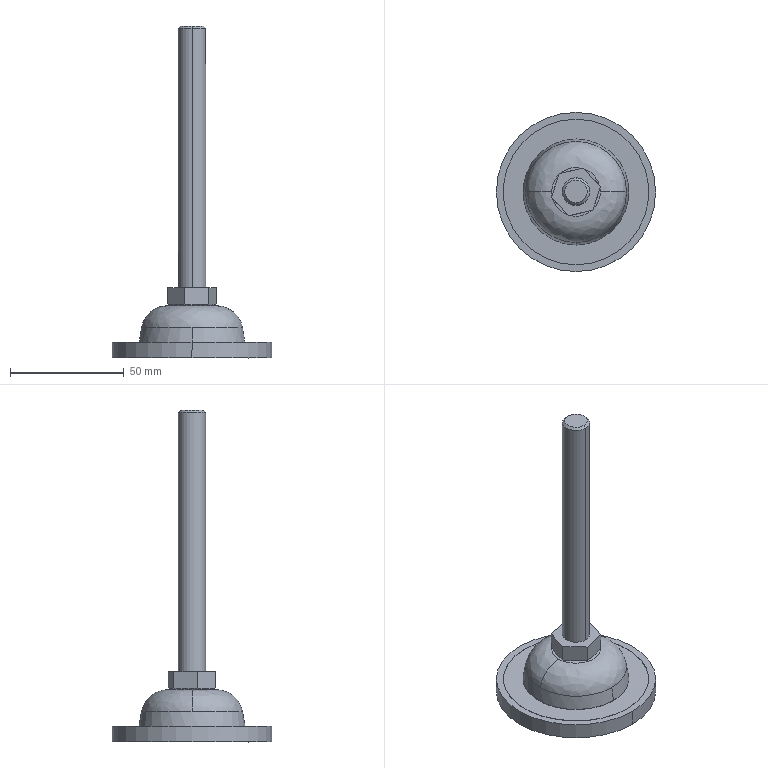Part | STEP file | HJM12-150 | 1 solid | 28 faces | box 70 x 70 x 146 mm | volume 64178 mm3 | plane 12 | cylinder 8 | cone 6 | spline 2 | commonest cylinder face diameters 12 x2 46.667 x2 64 x2 70 x2
STEP:
#1=CARTESIAN_POINT('',(1875.149,1272.903,-187.667));
#2=VERTEX_POINT('',#1);
#3=CARTESIAN_POINT('',(1852.937,1250.691,-187.667));
#4=VERTEX_POINT('',#3);
#5=CARTESIAN_POINT('',(1852.937,1272.903,-187.667));
#6=DIRECTION('',(0.,0.,-1.));
#7=DIRECTION('',(0.,1.,0.));
#8=AXIS2_PLACEMENT_3D('',#5,#6,#7);
#9=CIRCLE('',#8,22.212);
#10=EDGE_CURVE('',#2,#4,#9,.T.);
#11=ORIENTED_EDGE('',*,*,#10,.F.);
#12=CARTESIAN_POINT('',(1863.66,1272.903,-178.026));
#13=VERTEX_POINT('',#12);
#14=CARTESIAN_POINT('',(1863.66,1272.903,-189.693));
#15=DIRECTION('',(0.,-1.,0.));
#16=DIRECTION('',(1.,0.,0.));
#17=AXIS2_PLACEMENT_3D('',#14,#15,#16);
#18=CIRCLE('',#17,11.667);
#19=EDGE_CURVE('',#2,#13,#18,.T.);
#20=ORIENTED_EDGE('',*,*,#19,.T.);
#21=CARTESIAN_POINT('',(1855.305,1262.445,-178.026));
#22=VERTEX_POINT('',#21);
#23=CARTESIAN_POINT('',(1863.66,1272.903,-178.026));
#24=CARTESIAN_POINT('',(1863.66,1267.68,-178.026));
#25=CARTESIAN_POINT('',(1860.399,1263.599,-178.026));
#26=CARTESIAN_POINT('',(1855.305,1262.445,-178.026));
#27=(BOUNDED_CURVE()B_SPLINE_CURVE(3,(#23,#24,#25,#26),.UNSPECIFIED.,.F.,.T.)B_SPLINE_CURVE_WITH_KNOTS((4,4),(0.,1.),.UNSPECIFIED.)CURVE()GEOMETRIC_REPRESENTATION_ITEM()RATIONAL_B_SPLINE_CURVE((1.,0.8542,0.8542,1.))REPRESENTATION_ITEM(''));
#28=EDGE_CURVE('',#13,#22,#27,.T.);
#29=ORIENTED_EDGE('',*,*,#28,.T.);
#30=CARTESIAN_POINT('',(1850.185,1262.54,-178.026));
#31=VERTEX_POINT('',#30);
#32=CARTESIAN_POINT('',(1855.305,1262.445,-178.026));
#33=CARTESIAN_POINT('',(1853.607,1262.061,-178.026));
#34=CARTESIAN_POINT('',(1851.867,1262.093,-178.026));
#35=CARTESIAN_POINT('',(1850.185,1262.54,-178.026));
#36=(BOUNDED_CURVE()B_SPLINE_CURVE(3,(#32,#33,#34,#35),.UNSPECIFIED.,.F.,.T.)B_SPLINE_CURVE_WITH_KNOTS((4,4),(0.,1.),.UNSPECIFIED.)CURVE()GEOMETRIC_REPRESENTATION_ITEM()RATIONAL_B_SPLINE_CURVE((1.,0.9807,0.9807,1.))REPRESENTATION_ITEM(''));
#37=EDGE_CURVE('',#22,#31,#36,.T.);
#38=ORIENTED_EDGE('',*,*,#37,.T.);
#39=CARTESIAN_POINT('',(1842.214,1272.903,-178.026));
#40=VERTEX_POINT('',#39);
#41=CARTESIAN_POINT('',(1850.185,1262.54,-178.026));
#42=CARTESIAN_POINT('',(1849.053,1262.84,-178.026));
#43=CARTESIAN_POINT('',(1847.97,1263.328,-178.026));
#44=CARTESIAN_POINT('',(1846.02,1264.627,-178.026));
#45=CARTESIAN_POINT('',(1845.152,1265.437,-178.026));
#46=CARTESIAN_POINT('',(1843.723,1267.295,-178.026));
#47=CARTESIAN_POINT('',(1843.162,1268.341,-178.026));
#48=CARTESIAN_POINT('',(1842.408,1270.56,-178.026));
#49=CARTESIAN_POINT('',(1842.214,1271.731,-178.026));
#50=CARTESIAN_POINT('',(1842.214,1272.903,-178.026));
#51=B_SPLINE_CURVE_WITH_KNOTS('',3,(#41,#42,#43,#44,#45,#46,#47,#48,#49,#50),.UNSPECIFIED.,.F.,.F.,(4,2,2,2,4),(0.,0.25,0.5,0.75,1.),.UNSPECIFIED.);
#52=EDGE_CURVE('',#31,#40,#51,.T.);
#53=ORIENTED_EDGE('',*,*,#52,.T.);
#54=CARTESIAN_POINT('',(1830.725,1272.903,-187.667));
#55=VERTEX_POINT('',#54);
#56=CARTESIAN_POINT('',(1842.214,1272.903,-189.693));
#57=DIRECTION('',(0.,1.,0.));
#58=DIRECTION('',(-1.,0.,0.));
#59=AXIS2_PLACEMENT_3D('',#56,#57,#58);
#60=CIRCLE('',#59,11.667);
#61=EDGE_CURVE('',#55,#40,#60,.T.);
#62=ORIENTED_EDGE('',*,*,#61,.F.);
#63=CARTESIAN_POINT('',(1852.937,1272.903,-187.667));
#64=DIRECTION('',(0.,0.,-1.));
#65=DIRECTION('',(0.,1.,0.));
#66=AXIS2_PLACEMENT_3D('',#63,#64,#65);
#67=CIRCLE('',#66,22.212);
#68=EDGE_CURVE('',#4,#55,#67,.T.);
#69=ORIENTED_EDGE('',*,*,#68,.F.);
#70=EDGE_LOOP('',(#11,#20,#29,#38,#53,#62,#69));
#71=FACE_OUTER_BOUND('',#70,.T.);
#72=CARTESIAN_POINT('',(1875.149,1272.903,-187.667));
#73=CARTESIAN_POINT('',(1875.149,1228.479,-187.667));
#74=CARTESIAN_POINT('',(1830.725,1228.479,-187.667));
#75=CARTESIAN_POINT('',(1830.725,1272.903,-187.667));
#76=CARTESIAN_POINT('',(1874.12,1272.903,-181.834));
#77=CARTESIAN_POINT('',(1874.12,1230.536,-181.834));
#78=CARTESIAN_POINT('',(1831.754,1230.536,-181.834));
#79=CARTESIAN_POINT('',(1831.754,1272.903,-181.834));
#80=CARTESIAN_POINT('',(1869.583,1272.903,-178.026));
#81=CARTESIAN_POINT('',(1869.583,1239.611,-178.026));
#82=CARTESIAN_POINT('',(1836.291,1239.611,-178.026));
#83=CARTESIAN_POINT('',(1836.291,1272.903,-178.026));
#84=CARTESIAN_POINT('',(1863.66,1272.903,-178.026));
#85=CARTESIAN_POINT('',(1863.66,1251.458,-178.026));
#86=CARTESIAN_POINT('',(1842.214,1251.458,-178.026));
#87=CARTESIAN_POINT('',(1842.214,1272.903,-178.026));
#88=(BOUNDED_SURFACE()B_SPLINE_SURFACE(3,3,((#72,#73,#74,#75),(#76,#77,#78,#79),(#80,#81,#82,#83),(#84,#85,#86,#87)),.UNSPECIFIED.,.F.,.F.,.F.)B_SPLINE_SURFACE_WITH_KNOTS((4,4),(4,4),(0.,1.),(0.,1.),.UNSPECIFIED.)GEOMETRIC_REPRESENTATION_ITEM()RATIONAL_B_SPLINE_SURFACE(((1.,0.3333,0.3333,1.),(0.844,0.2813,0.2813,0.844),(0.844,0.2813,0.2813,0.844),(1.,0.3333,0.3333,1.)))REPRESENTATION_ITEM('')SURFACE());
#89=ADVANCED_FACE('',(#71),#88,.T.);
#90=CARTESIAN_POINT('',(1852.937,1237.903,-201.026));
#91=VERTEX_POINT('',#90);
#92=CARTESIAN_POINT('',(1852.937,1307.903,-201.026));
#93=VERTEX_POINT('',#92);
#94=CARTESIAN_POINT('',(1852.937,1272.903,-201.026));
#95=DIRECTION('',(0.,0.,1.));
#96=DIRECTION('',(0.,-1.,0.));
#97=AXIS2_PLACEMENT_3D('',#94,#95,#96);
#98=CIRCLE('',#97,35.);
#99=EDGE_CURVE('',#91,#93,#98,.T.);
#100=ORIENTED_EDGE('',*,*,#99,.T.);
#101=CARTESIAN_POINT('',(1852.937,1307.903,-194.026));
#102=VERTEX_POINT('',#101);
#103=CARTESIAN_POINT('',(1852.937,1307.903,-197.526));
#104=DIRECTION('',(0.,0.,1.));
#105=VECTOR('',#104,1000.);
#106=LINE('',#103,#105);
#107=EDGE_CURVE('',#93,#102,#106,.T.);
#108=ORIENTED_EDGE('',*,*,#107,.T.);
#109=CARTESIAN_POINT('',(1852.937,1237.903,-194.026));
#110=VERTEX_POINT('',#109);
#111=CARTESIAN_POINT('',(1852.937,1272.903,-194.026));
#112=DIRECTION('',(0.,0.,-1.));
#113=DIRECTION('',(0.,-1.,0.));
#114=AXIS2_PLACEMENT_3D('',#111,#112,#113);
#115=CIRCLE('',#114,35.);
#116=EDGE_CURVE('',#102,#110,#115,.T.);
#117=ORIENTED_EDGE('',*,*,#116,.T.);
#118=CARTESIAN_POINT('',(1852.937,1237.903,-197.526));
#119=DIRECTION('',(0.,0.,1.));
#120=VECTOR('',#119,1000.);
#121=LINE('',#118,#120);
#122=EDGE_CURVE('',#91,#110,#121,.T.);
#123=ORIENTED_EDGE('',*,*,#122,.F.);
#124=EDGE_LOOP('',(#100,#108,#117,#123));
#125=FACE_OUTER_BOUND('',#124,.T.);
#126=CARTESIAN_POINT('',(1852.937,1272.903,-197.526));
#127=DIRECTION('',(0.,0.,1.));
#128=DIRECTION('',(0.,-1.,0.));
#129=AXIS2_PLACEMENT_3D('',#126,#127,#128);
#130=CYLINDRICAL_SURFACE('',#129,35.);
#131=ADVANCED_FACE('',(#125),#130,.T.);
#132=CARTESIAN_POINT('',(1852.937,1304.903,-194.126));
#133=VERTEX_POINT('',#132);
#134=CARTESIAN_POINT('',(1852.937,1240.903,-194.126));
#135=VERTEX_POINT('',#134);
#136=CARTESIAN_POINT('',(1852.937,1272.903,-194.126));
#137=DIRECTION('',(0.,0.,1.));
#138=DIRECTION('',(0.,-1.,0.));
#139=AXIS2_PLACEMENT_3D('',#136,#137,#138);
#140=CIRCLE('',#139,32.);
#141=EDGE_CURVE('',#133,#135,#140,.T.);
#142=ORIENTED_EDGE('',*,*,#141,.F.);
#143=CARTESIAN_POINT('',(1852.937,1304.903,-194.026));
#144=VERTEX_POINT('',#143);
#145=CARTESIAN_POINT('',(1852.937,1304.903,-194.076));
#146=DIRECTION('',(0.,0.,1.));
#147=VECTOR('',#146,1000.);
#148=LINE('',#145,#147);
#149=EDGE_CURVE('',#133,#144,#148,.T.);
#150=ORIENTED_EDGE('',*,*,#149,.T.);
#151=CARTESIAN_POINT('',(1852.937,1240.903,-194.026));
#152=VERTEX_POINT('',#151);
#153=CARTESIAN_POINT('',(1852.937,1272.903,-194.026));
#154=DIRECTION('',(0.,0.,1.));
#155=DIRECTION('',(0.,-1.,0.));
#156=AXIS2_PLACEMENT_3D('',#153,#154,#155);
#157=CIRCLE('',#156,32.);
#158=EDGE_CURVE('',#144,#152,#157,.T.);
#159=ORIENTED_EDGE('',*,*,#158,.T.);
#160=CARTESIAN_POINT('',(1852.937,1240.903,-194.076));
#161=DIRECTION('',(0.,0.,1.));
#162=VECTOR('',#161,1000.);
#163=LINE('',#160,#162);
#164=EDGE_CURVE('',#135,#152,#163,.T.);
#165=ORIENTED_EDGE('',*,*,#164,.F.);
#166=EDGE_LOOP('',(#142,#150,#159,#165));
#167=FACE_OUTER_BOUND('',#166,.T.);
#168=CARTESIAN_POINT('',(1852.937,1272.903,-194.076));
#169=DIRECTION('',(0.,0.,1.));
#170=DIRECTION('',(0.,-1.,0.));
#171=AXIS2_PLACEMENT_3D('',#168,#169,#170);
#172=CYLINDRICAL_SURFACE('',#171,32.);
#173=ADVANCED_FACE('',(#167),#172,.F.);
#174=CARTESIAN_POINT('',(1852.937,1249.57,-194.126));
#175=VERTEX_POINT('',#174);
#176=CARTESIAN_POINT('',(1852.937,1296.236,-194.126));
#177=VERTEX_POINT('',#176);
#178=CARTESIAN_POINT('',(1852.937,1272.903,-194.126));
#179=DIRECTION('',(0.,0.,1.));
#180=DIRECTION('',(0.,-1.,0.));
#181=AXIS2_PLACEMENT_3D('',#178,#179,#180);
#182=CIRCLE('',#181,23.333);
#183=EDGE_CURVE('',#175,#177,#182,.T.);
#184=ORIENTED_EDGE('',*,*,#183,.T.);
#185=CARTESIAN_POINT('',(1852.937,1296.236,-194.026));
#186=VERTEX_POINT('',#185);
#187=CARTESIAN_POINT('',(1852.937,1296.236,-194.076));
#188=DIRECTION('',(0.,0.,1.));
#189=VECTOR('',#188,1000.);
#190=LINE('',#187,#189);
#191=EDGE_CURVE('',#177,#186,#190,.T.);
#192=ORIENTED_EDGE('',*,*,#191,.T.);
#193=CARTESIAN_POINT('',(1852.937,1249.57,-194.026));
#194=VERTEX_POINT('',#193);
#195=CARTESIAN_POINT('',(1852.937,1272.903,-194.026));
#196=DIRECTION('',(0.,0.,-1.));
#197=DIRECTION('',(0.,-1.,0.));
#198=AXIS2_PLACEMENT_3D('',#195,#196,#197);
#199=CIRCLE('',#198,23.333);
#200=EDGE_CURVE('',#186,#194,#199,.T.);
#201=ORIENTED_EDGE('',*,*,#200,.T.);
#202=CARTESIAN_POINT('',(1852.937,1249.57,-194.076));
#203=DIRECTION('',(0.,0.,1.));
#204=VECTOR('',#203,1000.);
#205=LINE('',#202,#204);
#206=EDGE_CURVE('',#175,#194,#205,.T.);
#207=ORIENTED_EDGE('',*,*,#206,.F.);
#208=EDGE_LOOP('',(#184,#192,#201,#207));
#209=FACE_OUTER_BOUND('',#208,.T.);
#210=CARTESIAN_POINT('',(1852.937,1272.903,-194.076));
#211=DIRECTION('',(0.,0.,1.));
#212=DIRECTION('',(0.,-1.,0.));
#213=AXIS2_PLACEMENT_3D('',#210,#211,#212);
#214=CYLINDRICAL_SURFACE('',#213,23.333);
#215=ADVANCED_FACE('',(#209),#214,.T.);
#216=CARTESIAN_POINT('',(1852.937,1295.115,-187.667));
#217=VERTEX_POINT('',#216);
#218=CARTESIAN_POINT('',(1852.937,1272.903,-187.667));
#219=DIRECTION('',(0.,0.,-1.));
#220=DIRECTION('',(0.,1.,0.));
#221=AXIS2_PLACEMENT_3D('',#218,#219,#220);
#222=CIRCLE('',#221,22.212);
#223=EDGE_CURVE('',#217,#2,#222,.T.);
#224=ORIENTED_EDGE('',*,*,#223,.T.);
#225=ORIENTED_EDGE('',*,*,#10,.T.);
#226=CARTESIAN_POINT('',(1852.937,1249.57,-194.026));
#227=DIRECTION('',(0.,-0.1736,-0.9848));
#228=VECTOR('',#227,1000.);
#229=LINE('',#226,#228);
#230=EDGE_CURVE('',#4,#194,#229,.T.);
#231=ORIENTED_EDGE('',*,*,#230,.T.);
#232=ORIENTED_EDGE('',*,*,#200,.F.);
#233=CARTESIAN_POINT('',(1852.937,1296.236,-194.026));
#234=DIRECTION('',(0.,0.1736,-0.9848));
#235=VECTOR('',#234,1000.);
#236=LINE('',#233,#235);
#237=EDGE_CURVE('',#217,#186,#236,.T.);
#238=ORIENTED_EDGE('',*,*,#237,.F.);
#239=EDGE_LOOP('',(#224,#225,#231,#232,#238));
#240=FACE_OUTER_BOUND('',#239,.T.);
#241=CARTESIAN_POINT('',(1852.937,1272.903,-194.026));
#242=DIRECTION('',(0.,0.,-1.));
#243=DIRECTION('',(0.,1.,0.));
#244=AXIS2_PLACEMENT_3D('',#241,#242,#243);
#245=CONICAL_SURFACE('',#244,23.333,0.1745);
#246=ADVANCED_FACE('',(#240),#245,.T.);
#247=CARTESIAN_POINT('',(1852.937,1264.903,-178.026));
#248=VERTEX_POINT('',#247);
#249=CARTESIAN_POINT('',(1852.937,1280.903,-178.026));
#250=VERTEX_POINT('',#249);
#251=CARTESIAN_POINT('',(1852.937,1272.903,-178.026));
#252=DIRECTION('',(0.,0.,1.));
#253=DIRECTION('',(0.,-1.,0.));
#254=AXIS2_PLACEMENT_3D('',#251,#252,#253);
#255=CIRCLE('',#254,8.);
#256=EDGE_CURVE('',#248,#250,#255,.T.);
#257=ORIENTED_EDGE('',*,*,#256,.T.);
#258=CARTESIAN_POINT('',(1852.937,1282.644,-177.577));
#259=VERTEX_POINT('',#258);
#260=CARTESIAN_POINT('',(1852.937,1283.891,-177.255));
#261=DIRECTION('',(0.,0.9683,0.2499));
#262=VECTOR('',#261,1000.);
#263=LINE('',#260,#262);
#264=EDGE_CURVE('',#250,#259,#263,.T.);
#265=ORIENTED_EDGE('',*,*,#264,.T.);
#266=CARTESIAN_POINT('',(1856.189,1283.38,-177.26));
#267=VERTEX_POINT('',#266);
#268=CARTESIAN_POINT('',(1852.937,1282.644,-177.577));
#269=CARTESIAN_POINT('',(1854.025,1282.89,-177.514));
#270=CARTESIAN_POINT('',(1855.108,1283.135,-177.403));
#271=CARTESIAN_POINT('',(1856.189,1283.38,-177.26));
#272=B_SPLINE_CURVE_WITH_KNOTS('',3,(#268,#269,#270,#271),.UNSPECIFIED.,.F.,.F.,(4,4),(0.,0.003349),.UNSPECIFIED.);
#273=EDGE_CURVE('',#259,#267,#272,.T.);
#274=ORIENTED_EDGE('',*,*,#273,.T.);
#275=CARTESIAN_POINT('',(1863.636,1275.325,-177.26));
#276=VERTEX_POINT('',#275);
#277=CARTESIAN_POINT('',(1856.189,1283.38,-177.26));
#278=CARTESIAN_POINT('',(1856.809,1282.709,-177.378));
#279=CARTESIAN_POINT('',(1857.43,1282.037,-177.474));
#280=CARTESIAN_POINT('',(1858.671,1280.695,-177.605));
#281=CARTESIAN_POINT('',(1859.912,1279.353,-177.674));
#282=CARTESIAN_POINT('',(1861.153,1278.01,-177.605));
#283=CARTESIAN_POINT('',(1862.395,1276.668,-177.474));
#284=CARTESIAN_POINT('',(1863.015,1275.997,-177.378));
#285=CARTESIAN_POINT('',(1863.636,1275.325,-177.26));
#286=B_SPLINE_CURVE_WITH_KNOTS('',3,(#277,#278,#279,#280,#281,#282,#283,#284,#285),.UNSPECIFIED.,.F.,.F.,(4,2,1,2,4),(0.,0.002742,0.005485,0.008227,0.01097),.UNSPECIFIED.);
#287=EDGE_CURVE('',#267,#276,#286,.T.);
#288=ORIENTED_EDGE('',*,*,#287,.T.);
#289=CARTESIAN_POINT('',(1860.384,1264.849,-177.26));
#290=VERTEX_POINT('',#289);
#291=CARTESIAN_POINT('',(1863.636,1275.325,-177.26));
#292=CARTESIAN_POINT('',(1863.365,1274.452,-177.378));
#293=CARTESIAN_POINT('',(1863.094,1273.579,-177.474));
#294=CARTESIAN_POINT('',(1862.552,1271.833,-177.605));
#295=CARTESIAN_POINT('',(1862.01,1270.087,-177.674));
#296=CARTESIAN_POINT('',(1861.468,1268.341,-177.605));
#297=CARTESIAN_POINT('',(1860.926,1266.595,-177.474));
#298=CARTESIAN_POINT('',(1860.655,1265.722,-177.378));
#299=CARTESIAN_POINT('',(1860.384,1264.849,-177.26));
#300=B_SPLINE_CURVE_WITH_KNOTS('',3,(#291,#292,#293,#294,#295,#296,#297,#298,#299),.UNSPECIFIED.,.F.,.F.,(4,2,1,2,4),(0.,0.002742,0.005485,0.008227,0.01097),.UNSPECIFIED.);
#301=EDGE_CURVE('',#276,#290,#300,.T.);
#302=ORIENTED_EDGE('',*,*,#301,.T.);
#303=CARTESIAN_POINT('',(1852.937,1263.163,-177.577));
#304=VERTEX_POINT('',#303);
#305=CARTESIAN_POINT('',(1860.384,1264.849,-177.26));
#306=CARTESIAN_POINT('',(1859.147,1264.569,-177.424));
#307=CARTESIAN_POINT('',(1857.909,1264.288,-177.545));
#308=CARTESIAN_POINT('',(1855.427,1263.726,-177.659));
#309=CARTESIAN_POINT('',(1854.183,1263.445,-177.65));
#310=CARTESIAN_POINT('',(1852.937,1263.163,-177.577));
#311=B_SPLINE_CURVE_WITH_KNOTS('',3,(#305,#306,#307,#308,#309,#310),.UNSPECIFIED.,.F.,.F.,(4,2,4),(0.,0.003821,0.007642),.UNSPECIFIED.);
#312=EDGE_CURVE('',#290,#304,#311,.T.);
#313=ORIENTED_EDGE('',*,*,#312,.T.);
#314=CARTESIAN_POINT('',(1852.937,1261.916,-177.255));
#315=DIRECTION('',(0.,-0.9683,0.2499));
#316=VECTOR('',#315,1000.);
#317=LINE('',#314,#316);
#318=EDGE_CURVE('',#248,#304,#317,.T.);
#319=ORIENTED_EDGE('',*,*,#318,.F.);
#320=EDGE_LOOP('',(#257,#265,#274,#288,#302,#313,#319));
#321=FACE_OUTER_BOUND('',#320,.T.);
#322=CARTESIAN_POINT('',(1852.937,1272.903,-177.255));
#323=DIRECTION('',(0.,0.,1.));
#324=DIRECTION('',(0.,-1.,0.));
#325=AXIS2_PLACEMENT_3D('',#322,#323,#324);
#326=CONICAL_SURFACE('',#325,10.987,1.318);
#327=ADVANCED_FACE('',(#321),#326,.T.);
#328=CARTESIAN_POINT('',(1852.937,1266.903,-170.026));
#329=VERTEX_POINT('',#328);
#330=CARTESIAN_POINT('',(1852.937,1278.903,-170.026));
#331=VERTEX_POINT('',#330);
#332=CARTESIAN_POINT('',(1852.937,1272.903,-170.026));
#333=DIRECTION('',(0.,0.,1.));
#334=DIRECTION('',(0.,-1.,0.));
#335=AXIS2_PLACEMENT_3D('',#332,#333,#334);
#336=CIRCLE('',#335,6.);
#337=EDGE_CURVE('',#329,#331,#336,.T.);
#338=ORIENTED_EDGE('',*,*,#337,.T.);
#339=CARTESIAN_POINT('',(1852.937,1278.903,-56.026));
#340=VERTEX_POINT('',#339);
#341=CARTESIAN_POINT('',(1852.937,1278.903,-133.063));
#342=DIRECTION('',(0.,0.,1.));
#343=VECTOR('',#342,1000.);
#344=LINE('',#341,#343);
#345=EDGE_CURVE('',#331,#340,#344,.T.);
#346=ORIENTED_EDGE('',*,*,#345,.T.);
#347=CARTESIAN_POINT('',(1852.937,1266.903,-56.026));
#348=VERTEX_POINT('',#347);
#349=CARTESIAN_POINT('',(1852.937,1272.903,-56.026));
#350=DIRECTION('',(0.,0.,-1.));
#351=DIRECTION('',(0.,-1.,0.));
#352=AXIS2_PLACEMENT_3D('',#349,#350,#351);
#353=CIRCLE('',#352,6.);
#354=EDGE_CURVE('',#340,#348,#353,.T.);
#355=ORIENTED_EDGE('',*,*,#354,.T.);
#356=CARTESIAN_POINT('',(1852.937,1266.903,-133.063));
#357=DIRECTION('',(0.,0.,1.));
#358=VECTOR('',#357,1000.);
#359=LINE('',#356,#358);
#360=EDGE_CURVE('',#329,#348,#359,.T.);
#361=ORIENTED_EDGE('',*,*,#360,.F.);
#362=EDGE_LOOP('',(#338,#346,#355,#361));
#363=FACE_OUTER_BOUND('',#362,.T.);
#364=CARTESIAN_POINT('',(1852.937,1272.903,-133.063));
#365=DIRECTION('',(0.,0.,1.));
#366=DIRECTION('',(0.,-1.,0.));
#367=AXIS2_PLACEMENT_3D('',#364,#365,#366);
#368=CYLINDRICAL_SURFACE('',#367,6.);
#369=ADVANCED_FACE('',(#363),#368,.T.);
#370=CARTESIAN_POINT('',(1852.937,1277.903,-55.026));
#371=VERTEX_POINT('',#370);
#372=CARTESIAN_POINT('',(1852.937,1267.903,-55.026));
#373=VERTEX_POINT('',#372);
#374=CARTESIAN_POINT('',(1852.937,1272.903,-55.026));
#375=DIRECTION('',(0.,0.,-1.));
#376=DIRECTION('',(0.,1.,0.));
#377=AXIS2_PLACEMENT_3D('',#374,#375,#376);
#378=CIRCLE('',#377,5.);
#379=EDGE_CURVE('',#371,#373,#378,.T.);
#380=ORIENTED_EDGE('',*,*,#379,.T.);
#381=CARTESIAN_POINT('',(1852.937,1266.903,-56.026));
#382=DIRECTION('',(0.,-0.7071,-0.7071));
#383=VECTOR('',#382,1000.);
#384=LINE('',#381,#383);
#385=EDGE_CURVE('',#373,#348,#384,.T.);
#386=ORIENTED_EDGE('',*,*,#385,.T.);
#387=ORIENTED_EDGE('',*,*,#354,.F.);
#388=CARTESIAN_POINT('',(1852.937,1278.903,-56.026));
#389=DIRECTION('',(0.,0.7071,-0.7071));
#390=VECTOR('',#389,1000.);
#391=LINE('',#388,#390);
#392=EDGE_CURVE('',#371,#340,#391,.T.);
#393=ORIENTED_EDGE('',*,*,#392,.F.);
#394=EDGE_LOOP('',(#380,#386,#387,#393));
#395=FACE_OUTER_BOUND('',#394,.T.);
#396=CARTESIAN_POINT('',(1852.937,1272.903,-56.026));
#397=DIRECTION('',(0.,0.,-1.));
#398=DIRECTION('',(0.,1.,0.));
#399=AXIS2_PLACEMENT_3D('',#396,#397,#398);
#400=CONICAL_SURFACE('',#399,6.,0.7854);
#401=ADVANCED_FACE('',(#395),#400,.T.);
#402=ORIENTED_EDGE('',*,*,#99,.F.);
#403=CARTESIAN_POINT('',(1852.937,1272.903,-201.026));
#404=DIRECTION('',(0.,0.,1.));
#405=DIRECTION('',(0.,-1.,0.));
#406=AXIS2_PLACEMENT_3D('',#403,#404,#405);
#407=CIRCLE('',#406,35.);
#408=EDGE_CURVE('',#93,#91,#407,.T.);
#409=ORIENTED_EDGE('',*,*,#408,.F.);
#410=EDGE_LOOP('',(#402,#409));
#411=FACE_OUTER_BOUND('',#410,.T.);
#412=CARTESIAN_POINT('',(1835.869,1269.039,-201.026));
#413=DIRECTION('',(0.,0.,1.));
#414=DIRECTION('',(0.,-1.,0.));
#415=AXIS2_PLACEMENT_3D('',#412,#413,#414);
#416=PLANE('',#415);
#417=ADVANCED_FACE('',(#411),#416,.F.);
#418=ORIENTED_EDGE('',*,*,#107,.F.);
#419=ORIENTED_EDGE('',*,*,#408,.T.);
#420=ORIENTED_EDGE('',*,*,#122,.T.);
#421=CARTESIAN_POINT('',(1852.937,1272.903,-194.026));
#422=DIRECTION('',(0.,0.,-1.));
#423=DIRECTION('',(0.,-1.,0.));
#424=AXIS2_PLACEMENT_3D('',#421,#422,#423);
#425=CIRCLE('',#424,35.);
#426=EDGE_CURVE('',#110,#102,#425,.T.);
#427=ORIENTED_EDGE('',*,*,#426,.T.);
#428=EDGE_LOOP('',(#418,#419,#420,#427));
#429=FACE_OUTER_BOUND('',#428,.T.);
#430=CARTESIAN_POINT('',(1852.937,1272.903,-197.526));
#431=DIRECTION('',(0.,0.,1.));
#432=DIRECTION('',(0.,-1.,0.));
#433=AXIS2_PLACEMENT_3D('',#430,#431,#432);
#434=CYLINDRICAL_SURFACE('',#433,35.);
#435=ADVANCED_FACE('',(#429),#434,.T.);
#436=ORIENTED_EDGE('',*,*,#426,.F.);
#437=ORIENTED_EDGE('',*,*,#116,.F.);
#438=EDGE_LOOP('',(#436,#437));
#439=FACE_OUTER_BOUND('',#438,.T.);
#440=CARTESIAN_POINT('',(1852.937,1272.903,-194.026));
#441=DIRECTION('',(0.,0.,1.));
#442=DIRECTION('',(0.,-1.,0.));
#443=AXIS2_PLACEMENT_3D('',#440,#441,#442);
#444=CIRCLE('',#443,32.);
#445=EDGE_CURVE('',#152,#144,#444,.T.);
#446=ORIENTED_EDGE('',*,*,#445,.F.);
#447=ORIENTED_EDGE('',*,*,#158,.F.);
#448=EDGE_LOOP('',(#446,#447));
#449=FACE_BOUND('',#448,.T.);
#450=CARTESIAN_POINT('',(1820.264,1265.506,-194.026));
#451=DIRECTION('',(0.,0.,-1.));
#452=DIRECTION('',(0.,1.,0.));
#453=AXIS2_PLACEMENT_3D('',#450,#451,#452);
#454=PLANE('',#453);
#455=ADVANCED_FACE('',(#439,#449),#454,.F.);
#456=ORIENTED_EDGE('',*,*,#149,.F.);
#457=CARTESIAN_POINT('',(1852.937,1272.903,-194.126));
#458=DIRECTION('',(0.,0.,1.));
#459=DIRECTION('',(0.,-1.,0.));
#460=AXIS2_PLACEMENT_3D('',#457,#458,#459);
#461=CIRCLE('',#460,32.);
#462=EDGE_CURVE('',#135,#133,#461,.T.);
#463=ORIENTED_EDGE('',*,*,#462,.F.);
#464=ORIENTED_EDGE('',*,*,#164,.T.);
#465=ORIENTED_EDGE('',*,*,#445,.T.);
#466=EDGE_LOOP('',(#456,#463,#464,#465));
#467=FACE_OUTER_BOUND('',#466,.T.);
#468=CARTESIAN_POINT('',(1852.937,1272.903,-194.076));
#469=DIRECTION('',(0.,0.,1.));
#470=DIRECTION('',(0.,-1.,0.));
#471=AXIS2_PLACEMENT_3D('',#468,#469,#470);
#472=CYLINDRICAL_SURFACE('',#471,32.);
#473=ADVANCED_FACE('',(#467),#472,.F.);
#474=ORIENTED_EDGE('',*,*,#462,.T.);
#475=ORIENTED_EDGE('',*,*,#141,.T.);
#476=EDGE_LOOP('',(#474,#475));
#477=FACE_OUTER_BOUND('',#476,.T.);
#478=ORIENTED_EDGE('',*,*,#183,.F.);
#479=CARTESIAN_POINT('',(1852.937,1272.903,-194.126));
#480=DIRECTION('',(0.,0.,1.));
#481=DIRECTION('',(0.,-1.,0.));
#482=AXIS2_PLACEMENT_3D('',#479,#480,#481);
#483=CIRCLE('',#482,23.333);
#484=EDGE_CURVE('',#177,#175,#483,.T.);
#485=ORIENTED_EDGE('',*,*,#484,.F.);
#486=EDGE_LOOP('',(#478,#485));
#487=FACE_BOUND('',#486,.T.);
#488=CARTESIAN_POINT('',(1825.953,1266.794,-194.126));
#489=DIRECTION('',(0.,0.,-1.));
#490=DIRECTION('',(0.,1.,0.));
#491=AXIS2_PLACEMENT_3D('',#488,#489,#490);
#492=PLANE('',#491);
#493=ADVANCED_FACE('',(#477,#487),#492,.F.);
#494=ORIENTED_EDGE('',*,*,#191,.F.);
#495=ORIENTED_EDGE('',*,*,#484,.T.);
#496=ORIENTED_EDGE('',*,*,#206,.T.);
#497=CARTESIAN_POINT('',(1852.937,1272.903,-194.026));
#498=DIRECTION('',(0.,0.,-1.));
#499=DIRECTION('',(0.,-1.,0.));
#500=AXIS2_PLACEMENT_3D('',#497,#498,#499);
#501=CIRCLE('',#500,23.333);
#502=EDGE_CURVE('',#194,#186,#501,.T.);
#503=ORIENTED_EDGE('',*,*,#502,.T.);
#504=EDGE_LOOP('',(#494,#495,#496,#503));
#505=FACE_OUTER_BOUND('',#504,.T.);
#506=CARTESIAN_POINT('',(1852.937,1272.903,-194.076));
#507=DIRECTION('',(0.,0.,1.));
#508=DIRECTION('',(0.,-1.,0.));
#509=AXIS2_PLACEMENT_3D('',#506,#507,#508);
#510=CYLINDRICAL_SURFACE('',#509,23.333);
#511=ADVANCED_FACE('',(#505),#510,.T.);
#512=ORIENTED_EDGE('',*,*,#230,.F.);
#513=ORIENTED_EDGE('',*,*,#68,.T.);
#514=CARTESIAN_POINT('',(1852.937,1272.903,-187.667));
#515=DIRECTION('',(0.,0.,-1.));
#516=DIRECTION('',(0.,1.,0.));
#517=AXIS2_PLACEMENT_3D('',#514,#515,#516);
#518=CIRCLE('',#517,22.212);
#519=EDGE_CURVE('',#55,#217,#518,.T.);
#520=ORIENTED_EDGE('',*,*,#519,.T.);
#521=ORIENTED_EDGE('',*,*,#237,.T.);
#522=ORIENTED_EDGE('',*,*,#502,.F.);
#523=EDGE_LOOP('',(#512,#513,#520,#521,#522));
#524=FACE_OUTER_BOUND('',#523,.T.);
#525=CARTESIAN_POINT('',(1852.937,1272.903,-194.026));
#526=DIRECTION('',(0.,0.,-1.));
#527=DIRECTION('',(0.,1.,0.));
#528=AXIS2_PLACEMENT_3D('',#525,#526,#527);
#529=CONICAL_SURFACE('',#528,23.333,0.1745);
#530=ADVANCED_FACE('',(#524),#529,.T.);
#531=ORIENTED_EDGE('',*,*,#19,.F.);
#532=ORIENTED_EDGE('',*,*,#223,.F.);
#533=ORIENTED_EDGE('',*,*,#519,.F.);
#534=ORIENTED_EDGE('',*,*,#61,.T.);
#535=CARTESIAN_POINT('',(1842.214,1272.903,-178.026));
#536=CARTESIAN_POINT('',(1842.214,1274.307,-178.026));
#537=CARTESIAN_POINT('',(1842.493,1275.71,-178.026));
#538=CARTESIAN_POINT('',(1843.567,1278.303,-178.026));
#539=CARTESIAN_POINT('',(1844.362,1279.493,-178.026));
#540=CARTESIAN_POINT('',(1846.347,1281.478,-178.026));
#541=CARTESIAN_POINT('',(1847.537,1282.273,-178.026));
#542=CARTESIAN_POINT('',(1850.13,1283.347,-178.026));
#543=CARTESIAN_POINT('',(1851.533,1283.626,-178.026));
#544=CARTESIAN_POINT('',(1854.341,1283.626,-178.026));
#545=CARTESIAN_POINT('',(1855.744,1283.347,-178.026));
#546=CARTESIAN_POINT('',(1858.337,1282.272,-178.026));
#547=CARTESIAN_POINT('',(1859.527,1281.478,-178.026));
#548=CARTESIAN_POINT('',(1861.512,1279.493,-178.026));
#549=CARTESIAN_POINT('',(1862.306,1278.303,-178.026));
#550=CARTESIAN_POINT('',(1863.381,1275.71,-178.026));
#551=CARTESIAN_POINT('',(1863.66,1274.307,-178.026));
#552=CARTESIAN_POINT('',(1863.66,1272.903,-178.026));
#553=B_SPLINE_CURVE_WITH_KNOTS('',3,(#535,#536,#537,#538,#539,#540,#541,#542,#543,#544,#545,#546,#547,#548,#549,#550,#551,#552),.UNSPECIFIED.,.F.,.F.,(4,2,2,2,2,2,2,2,4),(0.,0.125,0.25,0.375,0.5,0.625,0.75,0.875,1.),.UNSPECIFIED.);
#554=EDGE_CURVE('',#40,#13,#553,.T.);
#555=ORIENTED_EDGE('',*,*,#554,.T.);
#556=EDGE_LOOP('',(#531,#532,#533,#534,#555));
#557=FACE_OUTER_BOUND('',#556,.T.);
#558=CARTESIAN_POINT('',(1830.725,1272.903,-187.667));
#559=CARTESIAN_POINT('',(1830.725,1317.327,-187.667));
#560=CARTESIAN_POINT('',(1875.149,1317.327,-187.667));
#561=CARTESIAN_POINT('',(1875.149,1272.903,-187.667));
#562=CARTESIAN_POINT('',(1831.761,1272.903,-181.792));
#563=CARTESIAN_POINT('',(1831.761,1315.255,-181.792));
#564=CARTESIAN_POINT('',(1874.113,1315.255,-181.792));
#565=CARTESIAN_POINT('',(1874.113,1272.903,-181.792));
#566=CARTESIAN_POINT('',(1836.347,1272.903,-177.977));
#567=CARTESIAN_POINT('',(1836.347,1306.084,-177.977));
#568=CARTESIAN_POINT('',(1869.527,1306.084,-177.977));
#569=CARTESIAN_POINT('',(1869.527,1272.903,-177.977));
#570=CARTESIAN_POINT('',(1842.312,1272.903,-178.027));
#571=CARTESIAN_POINT('',(1842.312,1294.153,-178.027));
#572=CARTESIAN_POINT('',(1863.562,1294.153,-178.027));
#573=CARTESIAN_POINT('',(1863.562,1272.903,-178.027));
#574=(BOUNDED_SURFACE()B_SPLINE_SURFACE(3,3,((#558,#559,#560,#561),(#562,#563,#564,#565),(#566,#567,#568,#569),(#570,#571,#572,#573)),.UNSPECIFIED.,.F.,.F.,.F.)B_SPLINE_SURFACE_WITH_KNOTS((4,4),(4,4),(0.,1.),(0.,1.),.UNSPECIFIED.)GEOMETRIC_REPRESENTATION_ITEM()RATIONAL_B_SPLINE_SURFACE(((1.,0.3333,0.3333,1.),(0.8422,0.2807,0.2807,0.8422),(0.8422,0.2807,0.2807,0.8422),(1.,0.3333,0.3333,1.)))REPRESENTATION_ITEM('')SURFACE());
#575=ADVANCED_FACE('',(#557),#574,.T.);
#576=ORIENTED_EDGE('',*,*,#554,.F.);
#577=ORIENTED_EDGE('',*,*,#52,.F.);
#578=ORIENTED_EDGE('',*,*,#37,.F.);
#579=ORIENTED_EDGE('',*,*,#28,.F.);
#580=EDGE_LOOP('',(#576,#577,#578,#579));
#581=FACE_OUTER_BOUND('',#580,.T.);
#582=ORIENTED_EDGE('',*,*,#256,.F.);
#583=CARTESIAN_POINT('',(1852.937,1272.903,-178.026));
#584=DIRECTION('',(0.,0.,1.));
#585=DIRECTION('',(0.,-1.,0.));
#586=AXIS2_PLACEMENT_3D('',#583,#584,#585);
#587=CIRCLE('',#586,8.);
#588=EDGE_CURVE('',#250,#248,#587,.T.);
#589=ORIENTED_EDGE('',*,*,#588,.F.);
#590=EDGE_LOOP('',(#582,#589));
#591=FACE_BOUND('',#590,.T.);
#592=CARTESIAN_POINT('',(1843.807,1270.836,-178.026));
#593=DIRECTION('',(0.,0.,-1.));
#594=DIRECTION('',(0.,1.,0.));
#595=AXIS2_PLACEMENT_3D('',#592,#593,#594);
#596=PLANE('',#595);
#597=ADVANCED_FACE('',(#581,#591),#596,.F.);
#598=ORIENTED_EDGE('',*,*,#264,.F.);
#599=ORIENTED_EDGE('',*,*,#588,.T.);
#600=ORIENTED_EDGE('',*,*,#318,.T.);
#601=CARTESIAN_POINT('',(1849.685,1262.426,-177.26));
#602=VERTEX_POINT('',#601);
#603=CARTESIAN_POINT('',(1852.937,1263.163,-177.577));
#604=CARTESIAN_POINT('',(1851.849,1262.916,-177.514));
#605=CARTESIAN_POINT('',(1850.766,1262.671,-177.403));
#606=CARTESIAN_POINT('',(1849.685,1262.426,-177.26));
#607=B_SPLINE_CURVE_WITH_KNOTS('',3,(#603,#604,#605,#606),.UNSPECIFIED.,.F.,.F.,(4,4),(0.007642,0.01098),.UNSPECIFIED.);
#608=EDGE_CURVE('',#304,#602,#607,.T.);
#609=ORIENTED_EDGE('',*,*,#608,.T.);
#610=CARTESIAN_POINT('',(1842.238,1270.481,-177.26));
#611=VERTEX_POINT('',#610);
#612=CARTESIAN_POINT('',(1849.685,1262.426,-177.26));
#613=CARTESIAN_POINT('',(1849.065,1263.098,-177.378));
#614=CARTESIAN_POINT('',(1848.444,1263.769,-177.474));
#615=CARTESIAN_POINT('',(1847.203,1265.111,-177.605));
#616=CARTESIAN_POINT('',(1845.962,1266.454,-177.674));
#617=CARTESIAN_POINT('',(1844.721,1267.796,-177.605));
#618=CARTESIAN_POINT('',(1843.479,1269.138,-177.474));
#619=CARTESIAN_POINT('',(1842.859,1269.81,-177.378));
#620=CARTESIAN_POINT('',(1842.238,1270.481,-177.26));
#621=B_SPLINE_CURVE_WITH_KNOTS('',3,(#612,#613,#614,#615,#616,#617,#618,#619,#620),.UNSPECIFIED.,.F.,.F.,(4,2,1,2,4),(0.,0.002742,0.005485,0.008227,0.01097),.UNSPECIFIED.);
#622=EDGE_CURVE('',#602,#611,#621,.T.);
#623=ORIENTED_EDGE('',*,*,#622,.T.);
#624=CARTESIAN_POINT('',(1845.49,1280.957,-177.26));
#625=VERTEX_POINT('',#624);
#626=CARTESIAN_POINT('',(1842.238,1270.481,-177.26));
#627=CARTESIAN_POINT('',(1842.509,1271.354,-177.378));
#628=CARTESIAN_POINT('',(1842.78,1272.227,-177.474));
#629=CARTESIAN_POINT('',(1843.322,1273.973,-177.605));
#630=CARTESIAN_POINT('',(1843.864,1275.719,-177.674));
#631=CARTESIAN_POINT('',(1844.406,1277.465,-177.605));
#632=CARTESIAN_POINT('',(1844.948,1279.211,-177.474));
#633=CARTESIAN_POINT('',(1845.219,1280.084,-177.378));
#634=CARTESIAN_POINT('',(1845.49,1280.957,-177.26));
#635=B_SPLINE_CURVE_WITH_KNOTS('',3,(#626,#627,#628,#629,#630,#631,#632,#633,#634),.UNSPECIFIED.,.F.,.F.,(4,2,1,2,4),(0.,0.002742,0.005485,0.008227,0.01097),.UNSPECIFIED.);
#636=EDGE_CURVE('',#611,#625,#635,.T.);
#637=ORIENTED_EDGE('',*,*,#636,.T.);
#638=CARTESIAN_POINT('',(1845.49,1280.957,-177.26));
#639=CARTESIAN_POINT('',(1846.727,1281.237,-177.424));
#640=CARTESIAN_POINT('',(1847.965,1281.518,-177.545));
#641=CARTESIAN_POINT('',(1850.447,1282.08,-177.659));
#642=CARTESIAN_POINT('',(1851.691,1282.361,-177.65));
#643=CARTESIAN_POINT('',(1852.937,1282.644,-177.577));
#644=B_SPLINE_CURVE_WITH_KNOTS('',3,(#638,#639,#640,#641,#642,#643),.UNSPECIFIED.,.F.,.F.,(4,2,4),(-0.007674,-0.003837,0.),.UNSPECIFIED.);
#645=EDGE_CURVE('',#625,#259,#644,.T.);
#646=ORIENTED_EDGE('',*,*,#645,.T.);
#647=EDGE_LOOP('',(#598,#599,#600,#609,#623,#637,#646));
#648=FACE_OUTER_BOUND('',#647,.T.);
#649=CARTESIAN_POINT('',(1852.937,1272.903,-177.255));
#650=DIRECTION('',(0.,0.,1.));
#651=DIRECTION('',(0.,-1.,0.));
#652=AXIS2_PLACEMENT_3D('',#649,#650,#651);
#653=CONICAL_SURFACE('',#652,10.987,1.318);
#654=ADVANCED_FACE('',(#648),#653,.T.);
#655=CARTESIAN_POINT('',(1860.384,1264.849,-170.026));
#656=VERTEX_POINT('',#655);
#657=CARTESIAN_POINT('',(1849.685,1262.426,-170.026));
#658=VERTEX_POINT('',#657);
#659=CARTESIAN_POINT('',(1860.384,1264.849,-170.026));
#660=DIRECTION('',(-0.9753,-0.2208,0.));
#661=VECTOR('',#660,1000.);
#662=LINE('',#659,#661);
#663=EDGE_CURVE('',#656,#658,#662,.T.);
#664=ORIENTED_EDGE('',*,*,#663,.T.);
#665=CARTESIAN_POINT('',(1849.685,1262.426,-178.026));
#666=DIRECTION('',(0.,0.,-1.));
#667=VECTOR('',#666,1000.);
#668=LINE('',#665,#667);
#669=EDGE_CURVE('',#658,#602,#668,.T.);
#670=ORIENTED_EDGE('',*,*,#669,.T.);
#671=ORIENTED_EDGE('',*,*,#608,.F.);
#672=ORIENTED_EDGE('',*,*,#312,.F.);
#673=CARTESIAN_POINT('',(1860.384,1264.849,-178.026));
#674=DIRECTION('',(0.,0.,1.));
#675=VECTOR('',#674,1000.);
#676=LINE('',#673,#675);
#677=EDGE_CURVE('',#290,#656,#676,.T.);
#678=ORIENTED_EDGE('',*,*,#677,.T.);
#679=EDGE_LOOP('',(#664,#670,#671,#672,#678));
#680=FACE_OUTER_BOUND('',#679,.T.);
#681=CARTESIAN_POINT('',(1860.384,1264.849,-178.026));
#682=DIRECTION('',(0.2208,-0.9753,0.));
#683=DIRECTION('',(0.9753,0.2208,0.));
#684=AXIS2_PLACEMENT_3D('',#681,#682,#683);
#685=PLANE('',#684);
#686=ADVANCED_FACE('',(#680),#685,.T.);
#687=CARTESIAN_POINT('',(1863.636,1275.325,-170.026));
#688=VERTEX_POINT('',#687);
#689=CARTESIAN_POINT('',(1863.636,1275.325,-170.026));
#690=DIRECTION('',(-0.2964,-0.9551,0.));
#691=VECTOR('',#690,1000.);
#692=LINE('',#689,#691);
#693=EDGE_CURVE('',#688,#656,#692,.T.);
#694=ORIENTED_EDGE('',*,*,#693,.T.);
#695=ORIENTED_EDGE('',*,*,#677,.F.);
#696=ORIENTED_EDGE('',*,*,#301,.F.);
#697=CARTESIAN_POINT('',(1863.636,1275.325,-178.026));
#698=DIRECTION('',(0.,0.,1.));
#699=VECTOR('',#698,1000.);
#700=LINE('',#697,#699);
#701=EDGE_CURVE('',#276,#688,#700,.T.);
#702=ORIENTED_EDGE('',*,*,#701,.T.);
#703=EDGE_LOOP('',(#694,#695,#696,#702));
#704=FACE_OUTER_BOUND('',#703,.T.);
#705=CARTESIAN_POINT('',(1863.636,1275.325,-178.026));
#706=DIRECTION('',(0.9551,-0.2964,0.));
#707=DIRECTION('',(0.2964,0.9551,0.));
#708=AXIS2_PLACEMENT_3D('',#705,#706,#707);
#709=PLANE('',#708);
#710=ADVANCED_FACE('',(#704),#709,.T.);
#711=CARTESIAN_POINT('',(1856.189,1283.38,-170.026));
#712=VERTEX_POINT('',#711);
#713=CARTESIAN_POINT('',(1856.189,1283.38,-170.026));
#714=DIRECTION('',(0.6789,-0.7342,0.));
#715=VECTOR('',#714,1000.);
#716=LINE('',#713,#715);
#717=EDGE_CURVE('',#712,#688,#716,.T.);
#718=ORIENTED_EDGE('',*,*,#717,.T.);
#719=ORIENTED_EDGE('',*,*,#701,.F.);
#720=ORIENTED_EDGE('',*,*,#287,.F.);
#721=CARTESIAN_POINT('',(1856.189,1283.38,-178.026));
#722=DIRECTION('',(0.,0.,1.));
#723=VECTOR('',#722,1000.);
#724=LINE('',#721,#723);
#725=EDGE_CURVE('',#267,#712,#724,.T.);
#726=ORIENTED_EDGE('',*,*,#725,.T.);
#727=EDGE_LOOP('',(#718,#719,#720,#726));
#728=FACE_OUTER_BOUND('',#727,.T.);
#729=CARTESIAN_POINT('',(1856.189,1283.38,-178.026));
#730=DIRECTION('',(0.7342,0.6789,0.));
#731=DIRECTION('',(-0.6789,0.7342,0.));
#732=AXIS2_PLACEMENT_3D('',#729,#730,#731);
#733=PLANE('',#732);
#734=ADVANCED_FACE('',(#728),#733,.T.);
#735=CARTESIAN_POINT('',(1845.49,1280.957,-170.026));
#736=VERTEX_POINT('',#735);
#737=CARTESIAN_POINT('',(1845.49,1280.957,-170.026));
#738=DIRECTION('',(0.9753,0.2208,0.));
#739=VECTOR('',#738,1000.);
#740=LINE('',#737,#739);
#741=EDGE_CURVE('',#736,#712,#740,.T.);
#742=ORIENTED_EDGE('',*,*,#741,.T.);
#743=ORIENTED_EDGE('',*,*,#725,.F.);
#744=ORIENTED_EDGE('',*,*,#273,.F.);
#745=ORIENTED_EDGE('',*,*,#645,.F.);
#746=CARTESIAN_POINT('',(1845.49,1280.957,-178.026));
#747=DIRECTION('',(0.,0.,1.));
#748=VECTOR('',#747,1000.);
#749=LINE('',#746,#748);
#750=EDGE_CURVE('',#625,#736,#749,.T.);
#751=ORIENTED_EDGE('',*,*,#750,.T.);
#752=EDGE_LOOP('',(#742,#743,#744,#745,#751));
#753=FACE_OUTER_BOUND('',#752,.T.);
#754=CARTESIAN_POINT('',(1845.49,1280.957,-178.026));
#755=DIRECTION('',(-0.2208,0.9753,0.));
#756=DIRECTION('',(-0.9753,-0.2208,0.));
#757=AXIS2_PLACEMENT_3D('',#754,#755,#756);
#758=PLANE('',#757);
#759=ADVANCED_FACE('',(#753),#758,.T.);
#760=CARTESIAN_POINT('',(1842.238,1270.481,-170.026));
#761=VERTEX_POINT('',#760);
#762=CARTESIAN_POINT('',(1842.238,1270.481,-170.026));
#763=DIRECTION('',(0.2964,0.9551,0.));
#764=VECTOR('',#763,1000.);
#765=LINE('',#762,#764);
#766=EDGE_CURVE('',#761,#736,#765,.T.);
#767=ORIENTED_EDGE('',*,*,#766,.T.);
#768=ORIENTED_EDGE('',*,*,#750,.F.);
#769=ORIENTED_EDGE('',*,*,#636,.F.);
#770=CARTESIAN_POINT('',(1842.238,1270.481,-178.026));
#771=DIRECTION('',(0.,0.,1.));
#772=VECTOR('',#771,1000.);
#773=LINE('',#770,#772);
#774=EDGE_CURVE('',#611,#761,#773,.T.);
#775=ORIENTED_EDGE('',*,*,#774,.T.);
#776=EDGE_LOOP('',(#767,#768,#769,#775));
#777=FACE_OUTER_BOUND('',#776,.T.);
#778=CARTESIAN_POINT('',(1842.238,1270.481,-178.026));
#779=DIRECTION('',(-0.9551,0.2964,0.));
#780=DIRECTION('',(-0.2964,-0.9551,0.));
#781=AXIS2_PLACEMENT_3D('',#778,#779,#780);
#782=PLANE('',#781);
#783=ADVANCED_FACE('',(#777),#782,.T.);
#784=CARTESIAN_POINT('',(1849.685,1262.426,-170.026));
#785=DIRECTION('',(-0.6789,0.7342,0.));
#786=VECTOR('',#785,1000.);
#787=LINE('',#784,#786);
#788=EDGE_CURVE('',#658,#761,#787,.T.);
#789=ORIENTED_EDGE('',*,*,#788,.T.);
#790=ORIENTED_EDGE('',*,*,#774,.F.);
#791=ORIENTED_EDGE('',*,*,#622,.F.);
#792=ORIENTED_EDGE('',*,*,#669,.F.);
#793=EDGE_LOOP('',(#789,#790,#791,#792));
#794=FACE_OUTER_BOUND('',#793,.T.);
#795=CARTESIAN_POINT('',(1849.685,1262.426,-178.026));
#796=DIRECTION('',(-0.7342,-0.6789,0.));
#797=DIRECTION('',(0.6789,-0.7342,0.));
#798=AXIS2_PLACEMENT_3D('',#795,#796,#797);
#799=PLANE('',#798);
#800=ADVANCED_FACE('',(#794),#799,.T.);
#801=ORIENTED_EDGE('',*,*,#663,.F.);
#802=ORIENTED_EDGE('',*,*,#693,.F.);
#803=ORIENTED_EDGE('',*,*,#717,.F.);
#804=ORIENTED_EDGE('',*,*,#741,.F.);
#805=ORIENTED_EDGE('',*,*,#766,.F.);
#806=ORIENTED_EDGE('',*,*,#788,.F.);
#807=EDGE_LOOP('',(#801,#802,#803,#804,#805,#806));
#808=FACE_OUTER_BOUND('',#807,.T.);
#809=ORIENTED_EDGE('',*,*,#337,.F.);
#810=CARTESIAN_POINT('',(1852.937,1272.903,-170.026));
#811=DIRECTION('',(0.,0.,1.));
#812=DIRECTION('',(0.,-1.,0.));
#813=AXIS2_PLACEMENT_3D('',#810,#811,#812);
#814=CIRCLE('',#813,6.);
#815=EDGE_CURVE('',#331,#329,#814,.T.);
#816=ORIENTED_EDGE('',*,*,#815,.F.);
#817=EDGE_LOOP('',(#809,#816));
#818=FACE_BOUND('',#817,.T.);
#819=CARTESIAN_POINT('',(1844.22,1270.93,-170.026));
#820=DIRECTION('',(0.,0.,-1.));
#821=DIRECTION('',(0.,1.,0.));
#822=AXIS2_PLACEMENT_3D('',#819,#820,#821);
#823=PLANE('',#822);
#824=ADVANCED_FACE('',(#808,#818),#823,.F.);
#825=ORIENTED_EDGE('',*,*,#345,.F.);
#826=ORIENTED_EDGE('',*,*,#815,.T.);
#827=ORIENTED_EDGE('',*,*,#360,.T.);
#828=CARTESIAN_POINT('',(1852.937,1272.903,-56.026));
#829=DIRECTION('',(0.,0.,-1.));
#830=DIRECTION('',(0.,-1.,0.));
#831=AXIS2_PLACEMENT_3D('',#828,#829,#830);
#832=CIRCLE('',#831,6.);
#833=EDGE_CURVE('',#348,#340,#832,.T.);
#834=ORIENTED_EDGE('',*,*,#833,.T.);
#835=EDGE_LOOP('',(#825,#826,#827,#834));
#836=FACE_OUTER_BOUND('',#835,.T.);
#837=CARTESIAN_POINT('',(1852.937,1272.903,-133.063));
#838=DIRECTION('',(0.,0.,1.));
#839=DIRECTION('',(0.,-1.,0.));
#840=AXIS2_PLACEMENT_3D('',#837,#838,#839);
#841=CYLINDRICAL_SURFACE('',#840,6.);
#842=ADVANCED_FACE('',(#836),#841,.T.);
#843=ORIENTED_EDGE('',*,*,#385,.F.);
#844=CARTESIAN_POINT('',(1852.937,1272.903,-55.026));
#845=DIRECTION('',(0.,0.,-1.));
#846=DIRECTION('',(0.,1.,0.));
#847=AXIS2_PLACEMENT_3D('',#844,#845,#846);
#848=CIRCLE('',#847,5.);
#849=EDGE_CURVE('',#373,#371,#848,.T.);
#850=ORIENTED_EDGE('',*,*,#849,.T.);
#851=ORIENTED_EDGE('',*,*,#392,.T.);
#852=ORIENTED_EDGE('',*,*,#833,.F.);
#853=EDGE_LOOP('',(#843,#850,#851,#852));
#854=FACE_OUTER_BOUND('',#853,.T.);
#855=CARTESIAN_POINT('',(1852.937,1272.903,-56.026));
#856=DIRECTION('',(0.,0.,-1.));
#857=DIRECTION('',(0.,1.,0.));
#858=AXIS2_PLACEMENT_3D('',#855,#856,#857);
#859=CONICAL_SURFACE('',#858,6.,0.7854);
#860=ADVANCED_FACE('',(#854),#859,.T.);
#861=ORIENTED_EDGE('',*,*,#379,.F.);
#862=ORIENTED_EDGE('',*,*,#849,.F.);
#863=EDGE_LOOP('',(#861,#862));
#864=FACE_OUTER_BOUND('',#863,.T.);
#865=CARTESIAN_POINT('',(1852.937,1272.903,-55.026));
#866=DIRECTION('',(0.,0.,-1.));
#867=DIRECTION('',(0.,1.,0.));
#868=AXIS2_PLACEMENT_3D('',#865,#866,#867);
#869=PLANE('',#868);
#870=ADVANCED_FACE('',(#864),#869,.F.);
#871=CLOSED_SHELL('',(#89,#131,#173,#215,#246,#327,#369,#401,#417,#435,#455,#473,#493,#511,#530,#575,#597,#654,#686,#710,#734,#759,#783,#800,#824,#842,#860,#870));
#872=MANIFOLD_SOLID_BREP('',#871);
#873=CARTESIAN_POINT('',(0.,0.,0.));
#874=DIRECTION('',(0.,0.,1.));
#875=DIRECTION('',(1.,0.,0.));
#876=AXIS2_PLACEMENT_3D('',#873,#874,#875);
#877=(LENGTH_UNIT()NAMED_UNIT(*)SI_UNIT(.MILLI.,.METRE.));
#878=UNCERTAINTY_MEASURE_WITH_UNIT(LENGTH_MEASURE(0.00001),#877,'','');
#879=(NAMED_UNIT(*)PLANE_ANGLE_UNIT()SI_UNIT($,.RADIAN.));
#880=(NAMED_UNIT(*)SI_UNIT($,.STERADIAN.)SOLID_ANGLE_UNIT());
#881=(GEOMETRIC_REPRESENTATION_CONTEXT(3)GLOBAL_UNCERTAINTY_ASSIGNED_CONTEXT((#878))GLOBAL_UNIT_ASSIGNED_CONTEXT((#877,#879,#880))REPRESENTATION_CONTEXT('',''));
#882=ADVANCED_BREP_SHAPE_REPRESENTATION('',(#872,#876),#881);